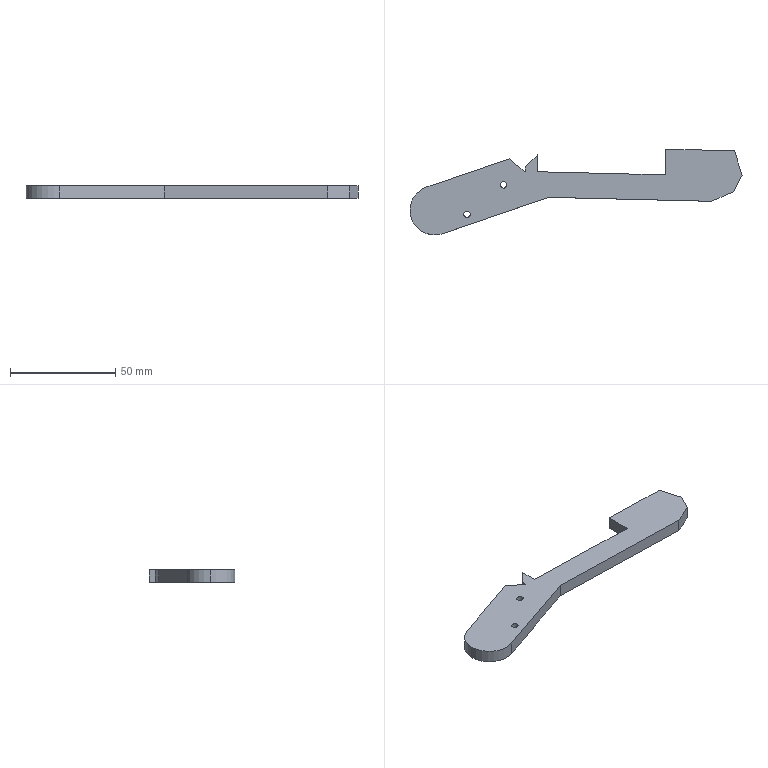Part | SolidWorks | features Chamfer 1, Extrusion 1, ICE 1 | 1 solid | 22 faces | box 157.426 x 40.732 x 6 mm | volume 17242 mm3 | plane 16 | cylinder 6 | commonest cylinder face diameters 3 x4 23.387 x2
STEP:
#1=CARTESIAN_POINT('',(-7.473,-11.857,6.));
#2=VERTEX_POINT('',#1);
#3=CARTESIAN_POINT('',(-4.473,-11.857,6.));
#4=VERTEX_POINT('',#3);
#5=CARTESIAN_POINT('',(-5.973,-11.857,6.));
#6=DIRECTION('',(0.,0.,1.));
#7=DIRECTION('',(1.,0.,0.));
#8=AXIS2_PLACEMENT_3D('',#5,#6,#7);
#9=CIRCLE('',#8,1.5);
#10=EDGE_CURVE('',#2,#4,#9,.T.);
#11=ORIENTED_EDGE('',*,*,#10,.T.);
#12=CARTESIAN_POINT('',(-4.473,-11.857,0.));
#13=VERTEX_POINT('',#12);
#14=CARTESIAN_POINT('',(-4.473,-11.857,6.));
#15=DIRECTION('',(0.,0.,-1.));
#16=VECTOR('',#15,1000.);
#17=LINE('',#14,#16);
#18=EDGE_CURVE('',#4,#13,#17,.T.);
#19=ORIENTED_EDGE('',*,*,#18,.T.);
#20=CARTESIAN_POINT('',(-7.473,-11.857,0.));
#21=VERTEX_POINT('',#20);
#22=CARTESIAN_POINT('',(-5.973,-11.857,0.));
#23=DIRECTION('',(0.,0.,1.));
#24=DIRECTION('',(1.,0.,0.));
#25=AXIS2_PLACEMENT_3D('',#22,#23,#24);
#26=CIRCLE('',#25,1.5);
#27=EDGE_CURVE('',#21,#13,#26,.T.);
#28=ORIENTED_EDGE('',*,*,#27,.F.);
#29=CARTESIAN_POINT('',(-7.473,-11.857,6.));
#30=DIRECTION('',(0.,0.,-1.));
#31=VECTOR('',#30,1000.);
#32=LINE('',#29,#31);
#33=EDGE_CURVE('',#2,#21,#32,.T.);
#34=ORIENTED_EDGE('',*,*,#33,.F.);
#35=EDGE_LOOP('',(#11,#19,#28,#34));
#36=FACE_OUTER_BOUND('',#35,.T.);
#37=CARTESIAN_POINT('',(-5.973,-11.857,6.));
#38=DIRECTION('',(0.,0.,-1.));
#39=DIRECTION('',(-1.,0.,0.));
#40=AXIS2_PLACEMENT_3D('',#37,#38,#39);
#41=CYLINDRICAL_SURFACE('',#40,1.5);
#42=ADVANCED_FACE('',(#36),#41,.F.);
#43=CARTESIAN_POINT('',(9.893,2.144,6.));
#44=VERTEX_POINT('',#43);
#45=CARTESIAN_POINT('',(12.893,2.144,6.));
#46=VERTEX_POINT('',#45);
#47=CARTESIAN_POINT('',(11.393,2.144,6.));
#48=DIRECTION('',(0.,0.,1.));
#49=DIRECTION('',(1.,0.,0.));
#50=AXIS2_PLACEMENT_3D('',#47,#48,#49);
#51=CIRCLE('',#50,1.5);
#52=EDGE_CURVE('',#44,#46,#51,.T.);
#53=ORIENTED_EDGE('',*,*,#52,.T.);
#54=CARTESIAN_POINT('',(12.893,2.144,0.));
#55=VERTEX_POINT('',#54);
#56=CARTESIAN_POINT('',(12.893,2.144,6.));
#57=DIRECTION('',(0.,0.,-1.));
#58=VECTOR('',#57,1000.);
#59=LINE('',#56,#58);
#60=EDGE_CURVE('',#46,#55,#59,.T.);
#61=ORIENTED_EDGE('',*,*,#60,.T.);
#62=CARTESIAN_POINT('',(9.893,2.144,0.));
#63=VERTEX_POINT('',#62);
#64=CARTESIAN_POINT('',(11.393,2.144,0.));
#65=DIRECTION('',(0.,0.,1.));
#66=DIRECTION('',(1.,0.,0.));
#67=AXIS2_PLACEMENT_3D('',#64,#65,#66);
#68=CIRCLE('',#67,1.5);
#69=EDGE_CURVE('',#63,#55,#68,.T.);
#70=ORIENTED_EDGE('',*,*,#69,.F.);
#71=CARTESIAN_POINT('',(9.893,2.144,6.));
#72=DIRECTION('',(0.,0.,-1.));
#73=VECTOR('',#72,1000.);
#74=LINE('',#71,#73);
#75=EDGE_CURVE('',#44,#63,#74,.T.);
#76=ORIENTED_EDGE('',*,*,#75,.F.);
#77=EDGE_LOOP('',(#53,#61,#70,#76));
#78=FACE_OUTER_BOUND('',#77,.T.);
#79=CARTESIAN_POINT('',(11.393,2.144,6.));
#80=DIRECTION('',(0.,0.,-1.));
#81=DIRECTION('',(-1.,0.,0.));
#82=AXIS2_PLACEMENT_3D('',#79,#80,#81);
#83=CYLINDRICAL_SURFACE('',#82,1.5);
#84=ADVANCED_FACE('',(#78),#83,.F.);
#85=CARTESIAN_POINT('',(-33.,-9.949,6.));
#86=VERTEX_POINT('',#85);
#87=CARTESIAN_POINT('',(-17.194,-20.895,6.));
#88=VERTEX_POINT('',#87);
#89=CARTESIAN_POINT('',(-21.306,-9.949,6.));
#90=DIRECTION('',(0.,0.,1.));
#91=DIRECTION('',(1.,0.,0.));
#92=AXIS2_PLACEMENT_3D('',#89,#90,#91);
#93=CIRCLE('',#92,11.693);
#94=EDGE_CURVE('',#86,#88,#93,.T.);
#95=ORIENTED_EDGE('',*,*,#94,.F.);
#96=CARTESIAN_POINT('',(-33.,-9.949,0.));
#97=VERTEX_POINT('',#96);
#98=CARTESIAN_POINT('',(-33.,-9.949,6.));
#99=DIRECTION('',(0.,0.,-1.));
#100=VECTOR('',#99,1000.);
#101=LINE('',#98,#100);
#102=EDGE_CURVE('',#86,#97,#101,.T.);
#103=ORIENTED_EDGE('',*,*,#102,.T.);
#104=CARTESIAN_POINT('',(-17.194,-20.895,0.));
#105=VERTEX_POINT('',#104);
#106=CARTESIAN_POINT('',(-21.306,-9.949,0.));
#107=DIRECTION('',(0.,0.,1.));
#108=DIRECTION('',(1.,0.,0.));
#109=AXIS2_PLACEMENT_3D('',#106,#107,#108);
#110=CIRCLE('',#109,11.693);
#111=EDGE_CURVE('',#97,#105,#110,.T.);
#112=ORIENTED_EDGE('',*,*,#111,.T.);
#113=CARTESIAN_POINT('',(-17.194,-20.895,6.));
#114=DIRECTION('',(0.,0.,-1.));
#115=VECTOR('',#114,1000.);
#116=LINE('',#113,#115);
#117=EDGE_CURVE('',#88,#105,#116,.T.);
#118=ORIENTED_EDGE('',*,*,#117,.F.);
#119=EDGE_LOOP('',(#95,#103,#112,#118));
#120=FACE_OUTER_BOUND('',#119,.T.);
#121=CARTESIAN_POINT('',(-21.306,-9.949,6.));
#122=DIRECTION('',(0.,0.,-1.));
#123=DIRECTION('',(-1.,0.,0.));
#124=AXIS2_PLACEMENT_3D('',#121,#122,#123);
#125=CYLINDRICAL_SURFACE('',#124,11.693);
#126=ADVANCED_FACE('',(#120),#125,.T.);
#127=CARTESIAN_POINT('',(21.751,8.497,6.));
#128=VERTEX_POINT('',#127);
#129=CARTESIAN_POINT('',(21.138,8.512,6.));
#130=VERTEX_POINT('',#129);
#131=CARTESIAN_POINT('',(87.993,6.887,6.));
#132=DIRECTION('',(-0.9997,0.02431,0.));
#133=VECTOR('',#132,1000.);
#134=LINE('',#131,#133);
#135=EDGE_CURVE('',#128,#130,#134,.T.);
#136=ORIENTED_EDGE('',*,*,#135,.F.);
#137=CARTESIAN_POINT('',(21.751,8.497,0.));
#138=VERTEX_POINT('',#137);
#139=CARTESIAN_POINT('',(21.751,8.497,-13.556));
#140=DIRECTION('',(0.,0.,1.));
#141=VECTOR('',#140,1000.);
#142=LINE('',#139,#141);
#143=EDGE_CURVE('',#138,#128,#142,.T.);
#144=ORIENTED_EDGE('',*,*,#143,.F.);
#145=CARTESIAN_POINT('',(21.138,8.512,0.));
#146=VERTEX_POINT('',#145);
#147=CARTESIAN_POINT('',(87.993,6.887,0.));
#148=DIRECTION('',(-0.9997,0.02431,0.));
#149=VECTOR('',#148,1000.);
#150=LINE('',#147,#149);
#151=EDGE_CURVE('',#138,#146,#150,.T.);
#152=ORIENTED_EDGE('',*,*,#151,.T.);
#153=CARTESIAN_POINT('',(21.138,8.512,6.));
#154=DIRECTION('',(0.,0.,-1.));
#155=VECTOR('',#154,1000.);
#156=LINE('',#153,#155);
#157=EDGE_CURVE('',#130,#146,#156,.T.);
#158=ORIENTED_EDGE('',*,*,#157,.F.);
#159=EDGE_LOOP('',(#136,#144,#152,#158));
#160=FACE_OUTER_BOUND('',#159,.T.);
#161=CARTESIAN_POINT('',(87.993,6.887,6.));
#162=DIRECTION('',(-0.02431,-0.9997,0.));
#163=DIRECTION('',(0.9997,-0.02431,0.));
#164=AXIS2_PLACEMENT_3D('',#161,#162,#163);
#165=PLANE('',#164);
#166=ADVANCED_FACE('',(#160),#165,.F.);
#167=ORIENTED_EDGE('',*,*,#52,.F.);
#168=CARTESIAN_POINT('',(11.393,2.144,6.));
#169=DIRECTION('',(0.,0.,1.));
#170=DIRECTION('',(1.,0.,0.));
#171=AXIS2_PLACEMENT_3D('',#168,#169,#170);
#172=CIRCLE('',#171,1.5);
#173=EDGE_CURVE('',#46,#44,#172,.T.);
#174=ORIENTED_EDGE('',*,*,#173,.F.);
#175=EDGE_LOOP('',(#167,#174));
#176=FACE_BOUND('',#175,.T.);
#177=CARTESIAN_POINT('',(27.349,8.361,6.));
#178=VERTEX_POINT('',#177);
#179=CARTESIAN_POINT('',(27.349,16.305,6.));
#180=VERTEX_POINT('',#179);
#181=CARTESIAN_POINT('',(27.349,20.571,6.));
#182=DIRECTION('',(0.,1.,0.));
#183=VECTOR('',#182,1000.);
#184=LINE('',#181,#183);
#185=EDGE_CURVE('',#178,#180,#184,.T.);
#186=ORIENTED_EDGE('',*,*,#185,.T.);
#187=CARTESIAN_POINT('',(21.751,10.707,6.));
#188=VERTEX_POINT('',#187);
#189=CARTESIAN_POINT('',(-10.106,-21.15,6.));
#190=DIRECTION('',(-0.7071,-0.7071,0.));
#191=VECTOR('',#190,1000.);
#192=LINE('',#189,#191);
#193=EDGE_CURVE('',#180,#188,#192,.T.);
#194=ORIENTED_EDGE('',*,*,#193,.T.);
#195=CARTESIAN_POINT('',(21.751,20.707,6.));
#196=DIRECTION('',(0.,-1.,0.));
#197=VECTOR('',#196,1000.);
#198=LINE('',#195,#197);
#199=EDGE_CURVE('',#188,#128,#198,.T.);
#200=ORIENTED_EDGE('',*,*,#199,.T.);
#201=ORIENTED_EDGE('',*,*,#135,.T.);
#202=CARTESIAN_POINT('',(14.082,14.527,6.));
#203=VERTEX_POINT('',#202);
#204=CARTESIAN_POINT('',(21.138,8.512,6.));
#205=DIRECTION('',(-0.761,0.6487,0.));
#206=VECTOR('',#205,1000.);
#207=LINE('',#204,#206);
#208=EDGE_CURVE('',#130,#203,#207,.T.);
#209=ORIENTED_EDGE('',*,*,#208,.T.);
#210=CARTESIAN_POINT('',(-25.419,0.9973,6.));
#211=VERTEX_POINT('',#210);
#212=CARTESIAN_POINT('',(14.082,14.527,6.));
#213=DIRECTION('',(-0.946,-0.324,0.));
#214=VECTOR('',#213,1000.);
#215=LINE('',#212,#214);
#216=EDGE_CURVE('',#203,#211,#215,.T.);
#217=ORIENTED_EDGE('',*,*,#216,.T.);
#218=CARTESIAN_POINT('',(-21.306,-9.949,6.));
#219=DIRECTION('',(0.,0.,1.));
#220=DIRECTION('',(1.,0.,0.));
#221=AXIS2_PLACEMENT_3D('',#218,#219,#220);
#222=CIRCLE('',#221,11.693);
#223=EDGE_CURVE('',#211,#86,#222,.T.);
#224=ORIENTED_EDGE('',*,*,#223,.T.);
#225=ORIENTED_EDGE('',*,*,#94,.T.);
#226=CARTESIAN_POINT('',(32.618,-3.77,6.));
#227=VERTEX_POINT('',#226);
#228=CARTESIAN_POINT('',(-17.194,-20.895,6.));
#229=DIRECTION('',(0.9457,0.3251,0.));
#230=VECTOR('',#229,1000.);
#231=LINE('',#228,#230);
#232=EDGE_CURVE('',#88,#227,#231,.T.);
#233=ORIENTED_EDGE('',*,*,#232,.T.);
#234=CARTESIAN_POINT('',(110.037,-5.653,6.));
#235=VERTEX_POINT('',#234);
#236=CARTESIAN_POINT('',(32.618,-3.77,6.));
#237=DIRECTION('',(0.9997,-0.02431,0.));
#238=VECTOR('',#237,1000.);
#239=LINE('',#236,#238);
#240=EDGE_CURVE('',#227,#235,#239,.T.);
#241=ORIENTED_EDGE('',*,*,#240,.T.);
#242=CARTESIAN_POINT('',(120.419,-1.071,6.));
#243=VERTEX_POINT('',#242);
#244=CARTESIAN_POINT('',(110.037,-5.653,6.));
#245=DIRECTION('',(0.9149,0.4038,0.));
#246=VECTOR('',#245,1000.);
#247=LINE('',#244,#246);
#248=EDGE_CURVE('',#235,#243,#247,.T.);
#249=ORIENTED_EDGE('',*,*,#248,.T.);
#250=CARTESIAN_POINT('',(124.426,6.719,6.));
#251=VERTEX_POINT('',#250);
#252=CARTESIAN_POINT('',(120.419,-1.071,6.));
#253=DIRECTION('',(0.4575,0.8892,0.));
#254=VECTOR('',#253,1000.);
#255=LINE('',#252,#254);
#256=EDGE_CURVE('',#243,#251,#255,.T.);
#257=ORIENTED_EDGE('',*,*,#256,.T.);
#258=CARTESIAN_POINT('',(120.89,18.297,6.));
#259=VERTEX_POINT('',#258);
#260=CARTESIAN_POINT('',(124.426,6.719,6.));
#261=DIRECTION('',(-0.2922,0.9564,0.));
#262=VECTOR('',#261,1000.);
#263=LINE('',#260,#262);
#264=EDGE_CURVE('',#251,#259,#263,.T.);
#265=ORIENTED_EDGE('',*,*,#264,.T.);
#266=CARTESIAN_POINT('',(88.29,19.089,6.));
#267=VERTEX_POINT('',#266);
#268=CARTESIAN_POINT('',(120.89,18.297,6.));
#269=DIRECTION('',(-0.9997,0.02431,0.));
#270=VECTOR('',#269,1000.);
#271=LINE('',#268,#270);
#272=EDGE_CURVE('',#259,#267,#271,.T.);
#273=ORIENTED_EDGE('',*,*,#272,.T.);
#274=CARTESIAN_POINT('',(87.993,6.887,6.));
#275=VERTEX_POINT('',#274);
#276=CARTESIAN_POINT('',(88.29,19.089,6.));
#277=DIRECTION('',(-0.02431,-0.9997,0.));
#278=VECTOR('',#277,1000.);
#279=LINE('',#276,#278);
#280=EDGE_CURVE('',#267,#275,#279,.T.);
#281=ORIENTED_EDGE('',*,*,#280,.T.);
#282=CARTESIAN_POINT('',(87.993,6.887,6.));
#283=DIRECTION('',(-0.9997,0.02431,0.));
#284=VECTOR('',#283,1000.);
#285=LINE('',#282,#284);
#286=EDGE_CURVE('',#275,#178,#285,.T.);
#287=ORIENTED_EDGE('',*,*,#286,.T.);
#288=EDGE_LOOP('',(#186,#194,#200,#201,#209,#217,#224,#225,#233,#241,#249,#257,#265,#273,#281,#287));
#289=FACE_OUTER_BOUND('',#288,.T.);
#290=ORIENTED_EDGE('',*,*,#10,.F.);
#291=CARTESIAN_POINT('',(-5.973,-11.857,6.));
#292=DIRECTION('',(0.,0.,1.));
#293=DIRECTION('',(1.,0.,0.));
#294=AXIS2_PLACEMENT_3D('',#291,#292,#293);
#295=CIRCLE('',#294,1.5);
#296=EDGE_CURVE('',#4,#2,#295,.T.);
#297=ORIENTED_EDGE('',*,*,#296,.F.);
#298=EDGE_LOOP('',(#290,#297));
#299=FACE_BOUND('',#298,.T.);
#300=CARTESIAN_POINT('',(-21.306,-9.949,6.));
#301=DIRECTION('',(0.,0.,1.));
#302=DIRECTION('',(1.,0.,0.));
#303=AXIS2_PLACEMENT_3D('',#300,#301,#302);
#304=PLANE('',#303);
#305=ADVANCED_FACE('',(#176,#289,#299),#304,.T.);
#306=CARTESIAN_POINT('',(21.751,10.707,0.));
#307=VERTEX_POINT('',#306);
#308=CARTESIAN_POINT('',(21.751,20.707,0.));
#309=DIRECTION('',(0.,1.,0.));
#310=VECTOR('',#309,1000.);
#311=LINE('',#308,#310);
#312=EDGE_CURVE('',#138,#307,#311,.T.);
#313=ORIENTED_EDGE('',*,*,#312,.T.);
#314=CARTESIAN_POINT('',(27.349,16.305,0.));
#315=VERTEX_POINT('',#314);
#316=CARTESIAN_POINT('',(31.514,20.47,0.));
#317=DIRECTION('',(0.7071,0.7071,0.));
#318=VECTOR('',#317,1000.);
#319=LINE('',#316,#318);
#320=EDGE_CURVE('',#307,#315,#319,.T.);
#321=ORIENTED_EDGE('',*,*,#320,.T.);
#322=CARTESIAN_POINT('',(27.349,8.361,0.));
#323=VERTEX_POINT('',#322);
#324=CARTESIAN_POINT('',(27.349,20.571,0.));
#325=DIRECTION('',(0.,-1.,0.));
#326=VECTOR('',#325,1000.);
#327=LINE('',#324,#326);
#328=EDGE_CURVE('',#315,#323,#327,.T.);
#329=ORIENTED_EDGE('',*,*,#328,.T.);
#330=CARTESIAN_POINT('',(87.993,6.887,0.));
#331=VERTEX_POINT('',#330);
#332=CARTESIAN_POINT('',(87.993,6.887,0.));
#333=DIRECTION('',(-0.9997,0.02431,0.));
#334=VECTOR('',#333,1000.);
#335=LINE('',#332,#334);
#336=EDGE_CURVE('',#331,#323,#335,.T.);
#337=ORIENTED_EDGE('',*,*,#336,.F.);
#338=CARTESIAN_POINT('',(88.29,19.089,0.));
#339=VERTEX_POINT('',#338);
#340=CARTESIAN_POINT('',(88.29,19.089,0.));
#341=DIRECTION('',(-0.02431,-0.9997,0.));
#342=VECTOR('',#341,1000.);
#343=LINE('',#340,#342);
#344=EDGE_CURVE('',#339,#331,#343,.T.);
#345=ORIENTED_EDGE('',*,*,#344,.F.);
#346=CARTESIAN_POINT('',(120.89,18.297,0.));
#347=VERTEX_POINT('',#346);
#348=CARTESIAN_POINT('',(120.89,18.297,0.));
#349=DIRECTION('',(-0.9997,0.02431,0.));
#350=VECTOR('',#349,1000.);
#351=LINE('',#348,#350);
#352=EDGE_CURVE('',#347,#339,#351,.T.);
#353=ORIENTED_EDGE('',*,*,#352,.F.);
#354=CARTESIAN_POINT('',(124.426,6.719,0.));
#355=VERTEX_POINT('',#354);
#356=CARTESIAN_POINT('',(124.426,6.719,0.));
#357=DIRECTION('',(-0.2922,0.9564,0.));
#358=VECTOR('',#357,1000.);
#359=LINE('',#356,#358);
#360=EDGE_CURVE('',#355,#347,#359,.T.);
#361=ORIENTED_EDGE('',*,*,#360,.F.);
#362=CARTESIAN_POINT('',(120.419,-1.071,0.));
#363=VERTEX_POINT('',#362);
#364=CARTESIAN_POINT('',(120.419,-1.071,0.));
#365=DIRECTION('',(0.4575,0.8892,0.));
#366=VECTOR('',#365,1000.);
#367=LINE('',#364,#366);
#368=EDGE_CURVE('',#363,#355,#367,.T.);
#369=ORIENTED_EDGE('',*,*,#368,.F.);
#370=CARTESIAN_POINT('',(110.037,-5.653,0.));
#371=VERTEX_POINT('',#370);
#372=CARTESIAN_POINT('',(110.037,-5.653,0.));
#373=DIRECTION('',(0.9149,0.4038,0.));
#374=VECTOR('',#373,1000.);
#375=LINE('',#372,#374);
#376=EDGE_CURVE('',#371,#363,#375,.T.);
#377=ORIENTED_EDGE('',*,*,#376,.F.);
#378=CARTESIAN_POINT('',(32.618,-3.77,0.));
#379=VERTEX_POINT('',#378);
#380=CARTESIAN_POINT('',(32.618,-3.77,0.));
#381=DIRECTION('',(0.9997,-0.02431,0.));
#382=VECTOR('',#381,1000.);
#383=LINE('',#380,#382);
#384=EDGE_CURVE('',#379,#371,#383,.T.);
#385=ORIENTED_EDGE('',*,*,#384,.F.);
#386=CARTESIAN_POINT('',(-17.194,-20.895,0.));
#387=DIRECTION('',(0.9457,0.3251,0.));
#388=VECTOR('',#387,1000.);
#389=LINE('',#386,#388);
#390=EDGE_CURVE('',#105,#379,#389,.T.);
#391=ORIENTED_EDGE('',*,*,#390,.F.);
#392=ORIENTED_EDGE('',*,*,#111,.F.);
#393=CARTESIAN_POINT('',(-25.419,0.9973,0.));
#394=VERTEX_POINT('',#393);
#395=CARTESIAN_POINT('',(-21.306,-9.949,0.));
#396=DIRECTION('',(0.,0.,1.));
#397=DIRECTION('',(1.,0.,0.));
#398=AXIS2_PLACEMENT_3D('',#395,#396,#397);
#399=CIRCLE('',#398,11.693);
#400=EDGE_CURVE('',#394,#97,#399,.T.);
#401=ORIENTED_EDGE('',*,*,#400,.F.);
#402=CARTESIAN_POINT('',(14.082,14.527,0.));
#403=VERTEX_POINT('',#402);
#404=CARTESIAN_POINT('',(14.082,14.527,0.));
#405=DIRECTION('',(-0.946,-0.324,0.));
#406=VECTOR('',#405,1000.);
#407=LINE('',#404,#406);
#408=EDGE_CURVE('',#403,#394,#407,.T.);
#409=ORIENTED_EDGE('',*,*,#408,.F.);
#410=CARTESIAN_POINT('',(21.138,8.512,0.));
#411=DIRECTION('',(-0.761,0.6487,0.));
#412=VECTOR('',#411,1000.);
#413=LINE('',#410,#412);
#414=EDGE_CURVE('',#146,#403,#413,.T.);
#415=ORIENTED_EDGE('',*,*,#414,.F.);
#416=ORIENTED_EDGE('',*,*,#151,.F.);
#417=EDGE_LOOP('',(#313,#321,#329,#337,#345,#353,#361,#369,#377,#385,#391,#392,#401,#409,#415,#416));
#418=FACE_OUTER_BOUND('',#417,.T.);
#419=ORIENTED_EDGE('',*,*,#69,.T.);
#420=CARTESIAN_POINT('',(11.393,2.144,0.));
#421=DIRECTION('',(0.,0.,1.));
#422=DIRECTION('',(1.,0.,0.));
#423=AXIS2_PLACEMENT_3D('',#420,#421,#422);
#424=CIRCLE('',#423,1.5);
#425=EDGE_CURVE('',#55,#63,#424,.T.);
#426=ORIENTED_EDGE('',*,*,#425,.T.);
#427=EDGE_LOOP('',(#419,#426));
#428=FACE_BOUND('',#427,.T.);
#429=ORIENTED_EDGE('',*,*,#27,.T.);
#430=CARTESIAN_POINT('',(-5.973,-11.857,0.));
#431=DIRECTION('',(0.,0.,1.));
#432=DIRECTION('',(1.,0.,0.));
#433=AXIS2_PLACEMENT_3D('',#430,#431,#432);
#434=CIRCLE('',#433,1.5);
#435=EDGE_CURVE('',#13,#21,#434,.T.);
#436=ORIENTED_EDGE('',*,*,#435,.T.);
#437=EDGE_LOOP('',(#429,#436));
#438=FACE_BOUND('',#437,.T.);
#439=CARTESIAN_POINT('',(-21.306,-9.949,0.));
#440=DIRECTION('',(0.,0.,1.));
#441=DIRECTION('',(1.,0.,0.));
#442=AXIS2_PLACEMENT_3D('',#439,#440,#441);
#443=PLANE('',#442);
#444=ADVANCED_FACE('',(#418,#428,#438),#443,.F.);
#445=ORIENTED_EDGE('',*,*,#336,.T.);
#446=CARTESIAN_POINT('',(27.349,8.361,-13.556));
#447=DIRECTION('',(0.,0.,1.));
#448=VECTOR('',#447,1000.);
#449=LINE('',#446,#448);
#450=EDGE_CURVE('',#323,#178,#449,.T.);
#451=ORIENTED_EDGE('',*,*,#450,.T.);
#452=ORIENTED_EDGE('',*,*,#286,.F.);
#453=CARTESIAN_POINT('',(87.993,6.887,6.));
#454=DIRECTION('',(0.,0.,-1.));
#455=VECTOR('',#454,1000.);
#456=LINE('',#453,#455);
#457=EDGE_CURVE('',#275,#331,#456,.T.);
#458=ORIENTED_EDGE('',*,*,#457,.T.);
#459=EDGE_LOOP('',(#445,#451,#452,#458));
#460=FACE_OUTER_BOUND('',#459,.T.);
#461=CARTESIAN_POINT('',(87.993,6.887,6.));
#462=DIRECTION('',(-0.02431,-0.9997,0.));
#463=DIRECTION('',(0.9997,-0.02431,0.));
#464=AXIS2_PLACEMENT_3D('',#461,#462,#463);
#465=PLANE('',#464);
#466=ADVANCED_FACE('',(#460),#465,.F.);
#467=ORIENTED_EDGE('',*,*,#414,.T.);
#468=CARTESIAN_POINT('',(14.082,14.527,6.));
#469=DIRECTION('',(0.,0.,-1.));
#470=VECTOR('',#469,1000.);
#471=LINE('',#468,#470);
#472=EDGE_CURVE('',#203,#403,#471,.T.);
#473=ORIENTED_EDGE('',*,*,#472,.F.);
#474=ORIENTED_EDGE('',*,*,#208,.F.);
#475=ORIENTED_EDGE('',*,*,#157,.T.);
#476=EDGE_LOOP('',(#467,#473,#474,#475));
#477=FACE_OUTER_BOUND('',#476,.T.);
#478=CARTESIAN_POINT('',(21.138,8.512,6.));
#479=DIRECTION('',(-0.6487,-0.761,0.));
#480=DIRECTION('',(0.761,-0.6487,0.));
#481=AXIS2_PLACEMENT_3D('',#478,#479,#480);
#482=PLANE('',#481);
#483=ADVANCED_FACE('',(#477),#482,.F.);
#484=ORIENTED_EDGE('',*,*,#408,.T.);
#485=CARTESIAN_POINT('',(-25.419,0.9973,6.));
#486=DIRECTION('',(0.,0.,-1.));
#487=VECTOR('',#486,1000.);
#488=LINE('',#485,#487);
#489=EDGE_CURVE('',#211,#394,#488,.T.);
#490=ORIENTED_EDGE('',*,*,#489,.F.);
#491=ORIENTED_EDGE('',*,*,#216,.F.);
#492=ORIENTED_EDGE('',*,*,#472,.T.);
#493=EDGE_LOOP('',(#484,#490,#491,#492));
#494=FACE_OUTER_BOUND('',#493,.T.);
#495=CARTESIAN_POINT('',(14.082,14.527,6.));
#496=DIRECTION('',(0.324,-0.946,0.));
#497=DIRECTION('',(0.946,0.324,0.));
#498=AXIS2_PLACEMENT_3D('',#495,#496,#497);
#499=PLANE('',#498);
#500=ADVANCED_FACE('',(#494),#499,.F.);
#501=ORIENTED_EDGE('',*,*,#102,.F.);
#502=ORIENTED_EDGE('',*,*,#223,.F.);
#503=ORIENTED_EDGE('',*,*,#489,.T.);
#504=ORIENTED_EDGE('',*,*,#400,.T.);
#505=EDGE_LOOP('',(#501,#502,#503,#504));
#506=FACE_OUTER_BOUND('',#505,.T.);
#507=CARTESIAN_POINT('',(-21.306,-9.949,6.));
#508=DIRECTION('',(0.,0.,-1.));
#509=DIRECTION('',(-1.,0.,0.));
#510=AXIS2_PLACEMENT_3D('',#507,#508,#509);
#511=CYLINDRICAL_SURFACE('',#510,11.693);
#512=ADVANCED_FACE('',(#506),#511,.T.);
#513=ORIENTED_EDGE('',*,*,#390,.T.);
#514=CARTESIAN_POINT('',(32.618,-3.77,6.));
#515=DIRECTION('',(0.,0.,-1.));
#516=VECTOR('',#515,1000.);
#517=LINE('',#514,#516);
#518=EDGE_CURVE('',#227,#379,#517,.T.);
#519=ORIENTED_EDGE('',*,*,#518,.F.);
#520=ORIENTED_EDGE('',*,*,#232,.F.);
#521=ORIENTED_EDGE('',*,*,#117,.T.);
#522=EDGE_LOOP('',(#513,#519,#520,#521));
#523=FACE_OUTER_BOUND('',#522,.T.);
#524=CARTESIAN_POINT('',(-17.194,-20.895,6.));
#525=DIRECTION('',(-0.3251,0.9457,0.));
#526=DIRECTION('',(-0.9457,-0.3251,0.));
#527=AXIS2_PLACEMENT_3D('',#524,#525,#526);
#528=PLANE('',#527);
#529=ADVANCED_FACE('',(#523),#528,.F.);
#530=ORIENTED_EDGE('',*,*,#384,.T.);
#531=CARTESIAN_POINT('',(110.037,-5.653,6.));
#532=DIRECTION('',(0.,0.,-1.));
#533=VECTOR('',#532,1000.);
#534=LINE('',#531,#533);
#535=EDGE_CURVE('',#235,#371,#534,.T.);
#536=ORIENTED_EDGE('',*,*,#535,.F.);
#537=ORIENTED_EDGE('',*,*,#240,.F.);
#538=ORIENTED_EDGE('',*,*,#518,.T.);
#539=EDGE_LOOP('',(#530,#536,#537,#538));
#540=FACE_OUTER_BOUND('',#539,.T.);
#541=CARTESIAN_POINT('',(32.618,-3.77,6.));
#542=DIRECTION('',(0.02431,0.9997,0.));
#543=DIRECTION('',(-0.9997,0.02431,0.));
#544=AXIS2_PLACEMENT_3D('',#541,#542,#543);
#545=PLANE('',#544);
#546=ADVANCED_FACE('',(#540),#545,.F.);
#547=ORIENTED_EDGE('',*,*,#376,.T.);
#548=CARTESIAN_POINT('',(120.419,-1.071,6.));
#549=DIRECTION('',(0.,0.,-1.));
#550=VECTOR('',#549,1000.);
#551=LINE('',#548,#550);
#552=EDGE_CURVE('',#243,#363,#551,.T.);
#553=ORIENTED_EDGE('',*,*,#552,.F.);
#554=ORIENTED_EDGE('',*,*,#248,.F.);
#555=ORIENTED_EDGE('',*,*,#535,.T.);
#556=EDGE_LOOP('',(#547,#553,#554,#555));
#557=FACE_OUTER_BOUND('',#556,.T.);
#558=CARTESIAN_POINT('',(110.037,-5.653,6.));
#559=DIRECTION('',(-0.4038,0.9149,0.));
#560=DIRECTION('',(-0.9149,-0.4038,0.));
#561=AXIS2_PLACEMENT_3D('',#558,#559,#560);
#562=PLANE('',#561);
#563=ADVANCED_FACE('',(#557),#562,.F.);
#564=ORIENTED_EDGE('',*,*,#368,.T.);
#565=CARTESIAN_POINT('',(124.426,6.719,6.));
#566=DIRECTION('',(0.,0.,-1.));
#567=VECTOR('',#566,1000.);
#568=LINE('',#565,#567);
#569=EDGE_CURVE('',#251,#355,#568,.T.);
#570=ORIENTED_EDGE('',*,*,#569,.F.);
#571=ORIENTED_EDGE('',*,*,#256,.F.);
#572=ORIENTED_EDGE('',*,*,#552,.T.);
#573=EDGE_LOOP('',(#564,#570,#571,#572));
#574=FACE_OUTER_BOUND('',#573,.T.);
#575=CARTESIAN_POINT('',(120.419,-1.071,6.));
#576=DIRECTION('',(-0.8892,0.4575,0.));
#577=DIRECTION('',(-0.4575,-0.8892,0.));
#578=AXIS2_PLACEMENT_3D('',#575,#576,#577);
#579=PLANE('',#578);
#580=ADVANCED_FACE('',(#574),#579,.F.);
#581=ORIENTED_EDGE('',*,*,#360,.T.);
#582=CARTESIAN_POINT('',(120.89,18.297,6.));
#583=DIRECTION('',(0.,0.,-1.));
#584=VECTOR('',#583,1000.);
#585=LINE('',#582,#584);
#586=EDGE_CURVE('',#259,#347,#585,.T.);
#587=ORIENTED_EDGE('',*,*,#586,.F.);
#588=ORIENTED_EDGE('',*,*,#264,.F.);
#589=ORIENTED_EDGE('',*,*,#569,.T.);
#590=EDGE_LOOP('',(#581,#587,#588,#589));
#591=FACE_OUTER_BOUND('',#590,.T.);
#592=CARTESIAN_POINT('',(124.426,6.719,6.));
#593=DIRECTION('',(-0.9564,-0.2922,0.));
#594=DIRECTION('',(0.2922,-0.9564,0.));
#595=AXIS2_PLACEMENT_3D('',#592,#593,#594);
#596=PLANE('',#595);
#597=ADVANCED_FACE('',(#591),#596,.F.);
#598=ORIENTED_EDGE('',*,*,#352,.T.);
#599=CARTESIAN_POINT('',(88.29,19.089,6.));
#600=DIRECTION('',(0.,0.,-1.));
#601=VECTOR('',#600,1000.);
#602=LINE('',#599,#601);
#603=EDGE_CURVE('',#267,#339,#602,.T.);
#604=ORIENTED_EDGE('',*,*,#603,.F.);
#605=ORIENTED_EDGE('',*,*,#272,.F.);
#606=ORIENTED_EDGE('',*,*,#586,.T.);
#607=EDGE_LOOP('',(#598,#604,#605,#606));
#608=FACE_OUTER_BOUND('',#607,.T.);
#609=CARTESIAN_POINT('',(120.89,18.297,6.));
#610=DIRECTION('',(-0.02431,-0.9997,0.));
#611=DIRECTION('',(0.9997,-0.02431,0.));
#612=AXIS2_PLACEMENT_3D('',#609,#610,#611);
#613=PLANE('',#612);
#614=ADVANCED_FACE('',(#608),#613,.F.);
#615=ORIENTED_EDGE('',*,*,#344,.T.);
#616=ORIENTED_EDGE('',*,*,#457,.F.);
#617=ORIENTED_EDGE('',*,*,#280,.F.);
#618=ORIENTED_EDGE('',*,*,#603,.T.);
#619=EDGE_LOOP('',(#615,#616,#617,#618));
#620=FACE_OUTER_BOUND('',#619,.T.);
#621=CARTESIAN_POINT('',(88.29,19.089,6.));
#622=DIRECTION('',(0.9997,-0.02431,0.));
#623=DIRECTION('',(0.02431,0.9997,0.));
#624=AXIS2_PLACEMENT_3D('',#621,#622,#623);
#625=PLANE('',#624);
#626=ADVANCED_FACE('',(#620),#625,.F.);
#627=ORIENTED_EDGE('',*,*,#60,.F.);
#628=ORIENTED_EDGE('',*,*,#173,.T.);
#629=ORIENTED_EDGE('',*,*,#75,.T.);
#630=ORIENTED_EDGE('',*,*,#425,.F.);
#631=EDGE_LOOP('',(#627,#628,#629,#630));
#632=FACE_OUTER_BOUND('',#631,.T.);
#633=CARTESIAN_POINT('',(11.393,2.144,6.));
#634=DIRECTION('',(0.,0.,-1.));
#635=DIRECTION('',(-1.,0.,0.));
#636=AXIS2_PLACEMENT_3D('',#633,#634,#635);
#637=CYLINDRICAL_SURFACE('',#636,1.5);
#638=ADVANCED_FACE('',(#632),#637,.F.);
#639=ORIENTED_EDGE('',*,*,#18,.F.);
#640=ORIENTED_EDGE('',*,*,#296,.T.);
#641=ORIENTED_EDGE('',*,*,#33,.T.);
#642=ORIENTED_EDGE('',*,*,#435,.F.);
#643=EDGE_LOOP('',(#639,#640,#641,#642));
#644=FACE_OUTER_BOUND('',#643,.T.);
#645=CARTESIAN_POINT('',(-5.973,-11.857,6.));
#646=DIRECTION('',(0.,0.,-1.));
#647=DIRECTION('',(-1.,0.,0.));
#648=AXIS2_PLACEMENT_3D('',#645,#646,#647);
#649=CYLINDRICAL_SURFACE('',#648,1.5);
#650=ADVANCED_FACE('',(#644),#649,.F.);
#651=ORIENTED_EDGE('',*,*,#199,.F.);
#652=CARTESIAN_POINT('',(21.751,10.707,-13.556));
#653=DIRECTION('',(0.,0.,-1.));
#654=VECTOR('',#653,1000.);
#655=LINE('',#652,#654);
#656=EDGE_CURVE('',#188,#307,#655,.T.);
#657=ORIENTED_EDGE('',*,*,#656,.T.);
#658=ORIENTED_EDGE('',*,*,#312,.F.);
#659=ORIENTED_EDGE('',*,*,#143,.T.);
#660=EDGE_LOOP('',(#651,#657,#658,#659));
#661=FACE_OUTER_BOUND('',#660,.T.);
#662=CARTESIAN_POINT('',(21.751,20.707,-13.556));
#663=DIRECTION('',(-1.,0.,0.));
#664=DIRECTION('',(0.,-1.,0.));
#665=AXIS2_PLACEMENT_3D('',#662,#663,#664);
#666=PLANE('',#665);
#667=ADVANCED_FACE('',(#661),#666,.T.);
#668=ORIENTED_EDGE('',*,*,#328,.F.);
#669=CARTESIAN_POINT('',(27.349,16.305,-13.556));
#670=DIRECTION('',(0.,0.,1.));
#671=VECTOR('',#670,1000.);
#672=LINE('',#669,#671);
#673=EDGE_CURVE('',#315,#180,#672,.T.);
#674=ORIENTED_EDGE('',*,*,#673,.T.);
#675=ORIENTED_EDGE('',*,*,#185,.F.);
#676=ORIENTED_EDGE('',*,*,#450,.F.);
#677=EDGE_LOOP('',(#668,#674,#675,#676));
#678=FACE_OUTER_BOUND('',#677,.T.);
#679=CARTESIAN_POINT('',(27.349,20.571,-13.556));
#680=DIRECTION('',(1.,0.,0.));
#681=DIRECTION('',(0.,1.,0.));
#682=AXIS2_PLACEMENT_3D('',#679,#680,#681);
#683=PLANE('',#682);
#684=ADVANCED_FACE('',(#678),#683,.T.);
#685=ORIENTED_EDGE('',*,*,#320,.F.);
#686=ORIENTED_EDGE('',*,*,#656,.F.);
#687=ORIENTED_EDGE('',*,*,#193,.F.);
#688=ORIENTED_EDGE('',*,*,#673,.F.);
#689=EDGE_LOOP('',(#685,#686,#687,#688));
#690=FACE_OUTER_BOUND('',#689,.T.);
#691=CARTESIAN_POINT('',(31.514,20.47,-13.556));
#692=DIRECTION('',(0.7071,-0.7071,0.));
#693=DIRECTION('',(0.,0.,1.));
#694=AXIS2_PLACEMENT_3D('',#691,#692,#693);
#695=PLANE('',#694);
#696=ADVANCED_FACE('',(#690),#695,.F.);
#697=CLOSED_SHELL('',(#42,#84,#126,#166,#305,#444,#466,#483,#500,#512,#529,#546,#563,#580,#597,#614,#626,#638,#650,#667,#684,#696));
#698=MANIFOLD_SOLID_BREP('',#697);
#699=CARTESIAN_POINT('',(0.,0.,0.));
#700=DIRECTION('',(0.,0.,1.));
#701=DIRECTION('',(1.,0.,0.));
#702=AXIS2_PLACEMENT_3D('',#699,#700,#701);
#703=(LENGTH_UNIT()NAMED_UNIT(*)SI_UNIT(.MILLI.,.METRE.));
#704=UNCERTAINTY_MEASURE_WITH_UNIT(LENGTH_MEASURE(0.00001),#703,'','');
#705=(NAMED_UNIT(*)PLANE_ANGLE_UNIT()SI_UNIT($,.RADIAN.));
#706=(NAMED_UNIT(*)SI_UNIT($,.STERADIAN.)SOLID_ANGLE_UNIT());
#707=(GEOMETRIC_REPRESENTATION_CONTEXT(3)GLOBAL_UNCERTAINTY_ASSIGNED_CONTEXT((#704))GLOBAL_UNIT_ASSIGNED_CONTEXT((#703,#705,#706))REPRESENTATION_CONTEXT('',''));
#708=ADVANCED_BREP_SHAPE_REPRESENTATION('',(#698,#702),#707);